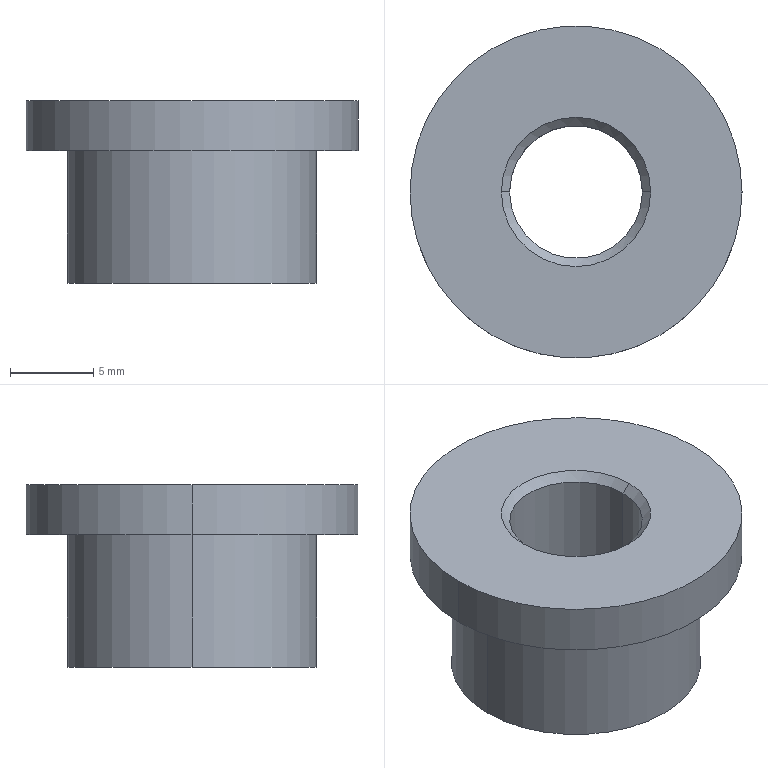Part | SolidWorks | features Chamfer 1, Extrusion 1, ICE 1 | 1 solid | 13 faces | box 20 x 20 x 11 mm | volume 1797 mm3 | cylinder 6 | cone 4 | plane 3 | commonest cylinder face diameters 8 x2 15 x2 20 x2
STEP:
#1=CARTESIAN_POINT('',(141.505,180.569,2.5));
#2=VERTEX_POINT('',#1);
#3=CARTESIAN_POINT('',(149.505,180.569,2.5));
#4=VERTEX_POINT('',#3);
#5=CARTESIAN_POINT('',(145.505,180.569,2.5));
#6=DIRECTION('',(0.,0.,1.));
#7=DIRECTION('',(1.,0.,0.));
#8=AXIS2_PLACEMENT_3D('',#5,#6,#7);
#9=CIRCLE('',#8,4.);
#10=EDGE_CURVE('',#2,#4,#9,.T.);
#11=ORIENTED_EDGE('',*,*,#10,.F.);
#12=CARTESIAN_POINT('',(141.005,180.569,3.));
#13=VERTEX_POINT('',#12);
#14=CARTESIAN_POINT('',(141.505,180.569,2.5));
#15=DIRECTION('',(-0.7071,0.,0.7071));
#16=VECTOR('',#15,1000.);
#17=LINE('',#14,#16);
#18=EDGE_CURVE('',#2,#13,#17,.T.);
#19=ORIENTED_EDGE('',*,*,#18,.T.);
#20=CARTESIAN_POINT('',(150.005,180.569,3.));
#21=VERTEX_POINT('',#20);
#22=CARTESIAN_POINT('',(145.505,180.569,3.));
#23=DIRECTION('',(0.,0.,-1.));
#24=DIRECTION('',(1.,0.,0.));
#25=AXIS2_PLACEMENT_3D('',#22,#23,#24);
#26=CIRCLE('',#25,4.5);
#27=EDGE_CURVE('',#21,#13,#26,.T.);
#28=ORIENTED_EDGE('',*,*,#27,.F.);
#29=CARTESIAN_POINT('',(149.505,180.569,2.5));
#30=DIRECTION('',(0.7071,0.,0.7071));
#31=VECTOR('',#30,1000.);
#32=LINE('',#29,#31);
#33=EDGE_CURVE('',#4,#21,#32,.T.);
#34=ORIENTED_EDGE('',*,*,#33,.F.);
#35=EDGE_LOOP('',(#11,#19,#28,#34));
#36=FACE_OUTER_BOUND('',#35,.T.);
#37=CARTESIAN_POINT('',(145.505,180.569,2.5));
#38=DIRECTION('',(0.,0.,1.));
#39=DIRECTION('',(1.,0.,0.));
#40=AXIS2_PLACEMENT_3D('',#37,#38,#39);
#41=CONICAL_SURFACE('',#40,4.,0.7854);
#42=ADVANCED_FACE('',(#36),#41,.F.);
#43=CARTESIAN_POINT('',(149.505,180.569,-7.5));
#44=VERTEX_POINT('',#43);
#45=CARTESIAN_POINT('',(141.505,180.569,-7.5));
#46=VERTEX_POINT('',#45);
#47=CARTESIAN_POINT('',(145.505,180.569,-7.5));
#48=DIRECTION('',(0.,0.,-1.));
#49=DIRECTION('',(1.,0.,0.));
#50=AXIS2_PLACEMENT_3D('',#47,#48,#49);
#51=CIRCLE('',#50,4.);
#52=EDGE_CURVE('',#44,#46,#51,.T.);
#53=ORIENTED_EDGE('',*,*,#52,.F.);
#54=CARTESIAN_POINT('',(150.005,180.569,-8.));
#55=VERTEX_POINT('',#54);
#56=CARTESIAN_POINT('',(149.505,180.569,-7.5));
#57=DIRECTION('',(0.7071,0.,-0.7071));
#58=VECTOR('',#57,1000.);
#59=LINE('',#56,#58);
#60=EDGE_CURVE('',#44,#55,#59,.T.);
#61=ORIENTED_EDGE('',*,*,#60,.T.);
#62=CARTESIAN_POINT('',(141.005,180.569,-8.));
#63=VERTEX_POINT('',#62);
#64=CARTESIAN_POINT('',(145.505,180.569,-8.));
#65=DIRECTION('',(0.,0.,1.));
#66=DIRECTION('',(1.,0.,0.));
#67=AXIS2_PLACEMENT_3D('',#64,#65,#66);
#68=CIRCLE('',#67,4.5);
#69=EDGE_CURVE('',#63,#55,#68,.T.);
#70=ORIENTED_EDGE('',*,*,#69,.F.);
#71=CARTESIAN_POINT('',(141.505,180.569,-7.5));
#72=DIRECTION('',(-0.7071,0.,-0.7071));
#73=VECTOR('',#72,1000.);
#74=LINE('',#71,#73);
#75=EDGE_CURVE('',#46,#63,#74,.T.);
#76=ORIENTED_EDGE('',*,*,#75,.F.);
#77=EDGE_LOOP('',(#53,#61,#70,#76));
#78=FACE_OUTER_BOUND('',#77,.T.);
#79=CARTESIAN_POINT('',(145.505,180.569,-7.5));
#80=DIRECTION('',(0.,0.,-1.));
#81=DIRECTION('',(-1.,0.,0.));
#82=AXIS2_PLACEMENT_3D('',#79,#80,#81);
#83=CONICAL_SURFACE('',#82,4.,0.7854);
#84=ADVANCED_FACE('',(#78),#83,.F.);
#85=CARTESIAN_POINT('',(155.505,180.569,3.));
#86=VERTEX_POINT('',#85);
#87=CARTESIAN_POINT('',(135.505,180.569,3.));
#88=VERTEX_POINT('',#87);
#89=CARTESIAN_POINT('',(145.505,180.569,3.));
#90=DIRECTION('',(0.,0.,1.));
#91=DIRECTION('',(1.,0.,0.));
#92=AXIS2_PLACEMENT_3D('',#89,#90,#91);
#93=CIRCLE('',#92,10.);
#94=EDGE_CURVE('',#86,#88,#93,.T.);
#95=ORIENTED_EDGE('',*,*,#94,.F.);
#96=CARTESIAN_POINT('',(155.505,180.569,0.));
#97=VERTEX_POINT('',#96);
#98=CARTESIAN_POINT('',(155.505,180.569,3.));
#99=DIRECTION('',(0.,0.,-1.));
#100=VECTOR('',#99,1000.);
#101=LINE('',#98,#100);
#102=EDGE_CURVE('',#86,#97,#101,.T.);
#103=ORIENTED_EDGE('',*,*,#102,.T.);
#104=CARTESIAN_POINT('',(135.505,180.569,0.));
#105=VERTEX_POINT('',#104);
#106=CARTESIAN_POINT('',(145.505,180.569,0.));
#107=DIRECTION('',(0.,0.,1.));
#108=DIRECTION('',(1.,0.,0.));
#109=AXIS2_PLACEMENT_3D('',#106,#107,#108);
#110=CIRCLE('',#109,10.);
#111=EDGE_CURVE('',#97,#105,#110,.T.);
#112=ORIENTED_EDGE('',*,*,#111,.T.);
#113=CARTESIAN_POINT('',(135.505,180.569,3.));
#114=DIRECTION('',(0.,0.,-1.));
#115=VECTOR('',#114,1000.);
#116=LINE('',#113,#115);
#117=EDGE_CURVE('',#88,#105,#116,.T.);
#118=ORIENTED_EDGE('',*,*,#117,.F.);
#119=EDGE_LOOP('',(#95,#103,#112,#118));
#120=FACE_OUTER_BOUND('',#119,.T.);
#121=CARTESIAN_POINT('',(145.505,180.569,3.));
#122=DIRECTION('',(0.,0.,-1.));
#123=DIRECTION('',(-1.,0.,0.));
#124=AXIS2_PLACEMENT_3D('',#121,#122,#123);
#125=CYLINDRICAL_SURFACE('',#124,10.);
#126=ADVANCED_FACE('',(#120),#125,.T.);
#127=ORIENTED_EDGE('',*,*,#52,.T.);
#128=CARTESIAN_POINT('',(141.505,180.569,-29.213));
#129=DIRECTION('',(0.,0.,1.));
#130=VECTOR('',#129,1000.);
#131=LINE('',#128,#130);
#132=EDGE_CURVE('',#46,#2,#131,.T.);
#133=ORIENTED_EDGE('',*,*,#132,.T.);
#134=ORIENTED_EDGE('',*,*,#10,.T.);
#135=CARTESIAN_POINT('',(149.505,180.569,-29.213));
#136=DIRECTION('',(0.,0.,1.));
#137=VECTOR('',#136,1000.);
#138=LINE('',#135,#137);
#139=EDGE_CURVE('',#44,#4,#138,.T.);
#140=ORIENTED_EDGE('',*,*,#139,.F.);
#141=EDGE_LOOP('',(#127,#133,#134,#140));
#142=FACE_OUTER_BOUND('',#141,.T.);
#143=CARTESIAN_POINT('',(145.505,180.569,-29.213));
#144=DIRECTION('',(0.,0.,1.));
#145=DIRECTION('',(1.,0.,0.));
#146=AXIS2_PLACEMENT_3D('',#143,#144,#145);
#147=CYLINDRICAL_SURFACE('',#146,4.);
#148=ADVANCED_FACE('',(#142),#147,.F.);
#149=CARTESIAN_POINT('',(138.005,180.569,-8.));
#150=VERTEX_POINT('',#149);
#151=CARTESIAN_POINT('',(153.005,180.569,-8.));
#152=VERTEX_POINT('',#151);
#153=CARTESIAN_POINT('',(145.505,180.569,-8.));
#154=DIRECTION('',(0.,0.,-1.));
#155=DIRECTION('',(1.,0.,0.));
#156=AXIS2_PLACEMENT_3D('',#153,#154,#155);
#157=CIRCLE('',#156,7.5);
#158=EDGE_CURVE('',#150,#152,#157,.T.);
#159=ORIENTED_EDGE('',*,*,#158,.F.);
#160=CARTESIAN_POINT('',(138.005,180.569,0.));
#161=VERTEX_POINT('',#160);
#162=CARTESIAN_POINT('',(138.005,180.569,-29.213));
#163=DIRECTION('',(0.,0.,1.));
#164=VECTOR('',#163,1000.);
#165=LINE('',#162,#164);
#166=EDGE_CURVE('',#150,#161,#165,.T.);
#167=ORIENTED_EDGE('',*,*,#166,.T.);
#168=CARTESIAN_POINT('',(153.005,180.569,0.));
#169=VERTEX_POINT('',#168);
#170=CARTESIAN_POINT('',(145.505,180.569,0.));
#171=DIRECTION('',(0.,0.,1.));
#172=DIRECTION('',(1.,0.,0.));
#173=AXIS2_PLACEMENT_3D('',#170,#171,#172);
#174=CIRCLE('',#173,7.5);
#175=EDGE_CURVE('',#169,#161,#174,.T.);
#176=ORIENTED_EDGE('',*,*,#175,.F.);
#177=CARTESIAN_POINT('',(153.005,180.569,-29.213));
#178=DIRECTION('',(0.,0.,1.));
#179=VECTOR('',#178,1000.);
#180=LINE('',#177,#179);
#181=EDGE_CURVE('',#152,#169,#180,.T.);
#182=ORIENTED_EDGE('',*,*,#181,.F.);
#183=EDGE_LOOP('',(#159,#167,#176,#182));
#184=FACE_OUTER_BOUND('',#183,.T.);
#185=CARTESIAN_POINT('',(145.505,180.569,-29.213));
#186=DIRECTION('',(0.,0.,1.));
#187=DIRECTION('',(1.,0.,0.));
#188=AXIS2_PLACEMENT_3D('',#185,#186,#187);
#189=CYLINDRICAL_SURFACE('',#188,7.5);
#190=ADVANCED_FACE('',(#184),#189,.T.);
#191=ORIENTED_EDGE('',*,*,#166,.F.);
#192=CARTESIAN_POINT('',(145.505,180.569,-8.));
#193=DIRECTION('',(0.,0.,-1.));
#194=DIRECTION('',(1.,0.,0.));
#195=AXIS2_PLACEMENT_3D('',#192,#193,#194);
#196=CIRCLE('',#195,7.5);
#197=EDGE_CURVE('',#152,#150,#196,.T.);
#198=ORIENTED_EDGE('',*,*,#197,.F.);
#199=ORIENTED_EDGE('',*,*,#181,.T.);
#200=CARTESIAN_POINT('',(145.505,180.569,0.));
#201=DIRECTION('',(0.,0.,1.));
#202=DIRECTION('',(1.,0.,0.));
#203=AXIS2_PLACEMENT_3D('',#200,#201,#202);
#204=CIRCLE('',#203,7.5);
#205=EDGE_CURVE('',#161,#169,#204,.T.);
#206=ORIENTED_EDGE('',*,*,#205,.F.);
#207=EDGE_LOOP('',(#191,#198,#199,#206));
#208=FACE_OUTER_BOUND('',#207,.T.);
#209=CARTESIAN_POINT('',(145.505,180.569,-29.213));
#210=DIRECTION('',(0.,0.,1.));
#211=DIRECTION('',(1.,0.,0.));
#212=AXIS2_PLACEMENT_3D('',#209,#210,#211);
#213=CYLINDRICAL_SURFACE('',#212,7.5);
#214=ADVANCED_FACE('',(#208),#213,.T.);
#215=ORIENTED_EDGE('',*,*,#132,.F.);
#216=CARTESIAN_POINT('',(145.505,180.569,-7.5));
#217=DIRECTION('',(0.,0.,-1.));
#218=DIRECTION('',(1.,0.,0.));
#219=AXIS2_PLACEMENT_3D('',#216,#217,#218);
#220=CIRCLE('',#219,4.);
#221=EDGE_CURVE('',#46,#44,#220,.T.);
#222=ORIENTED_EDGE('',*,*,#221,.T.);
#223=ORIENTED_EDGE('',*,*,#139,.T.);
#224=CARTESIAN_POINT('',(145.505,180.569,2.5));
#225=DIRECTION('',(0.,0.,1.));
#226=DIRECTION('',(1.,0.,0.));
#227=AXIS2_PLACEMENT_3D('',#224,#225,#226);
#228=CIRCLE('',#227,4.);
#229=EDGE_CURVE('',#4,#2,#228,.T.);
#230=ORIENTED_EDGE('',*,*,#229,.T.);
#231=EDGE_LOOP('',(#215,#222,#223,#230));
#232=FACE_OUTER_BOUND('',#231,.T.);
#233=CARTESIAN_POINT('',(145.505,180.569,-29.213));
#234=DIRECTION('',(0.,0.,1.));
#235=DIRECTION('',(1.,0.,0.));
#236=AXIS2_PLACEMENT_3D('',#233,#234,#235);
#237=CYLINDRICAL_SURFACE('',#236,4.);
#238=ADVANCED_FACE('',(#232),#237,.F.);
#239=ORIENTED_EDGE('',*,*,#69,.T.);
#240=CARTESIAN_POINT('',(145.505,180.569,-8.));
#241=DIRECTION('',(0.,0.,1.));
#242=DIRECTION('',(1.,0.,0.));
#243=AXIS2_PLACEMENT_3D('',#240,#241,#242);
#244=CIRCLE('',#243,4.5);
#245=EDGE_CURVE('',#55,#63,#244,.T.);
#246=ORIENTED_EDGE('',*,*,#245,.T.);
#247=EDGE_LOOP('',(#239,#246));
#248=FACE_BOUND('',#247,.T.);
#249=ORIENTED_EDGE('',*,*,#197,.T.);
#250=ORIENTED_EDGE('',*,*,#158,.T.);
#251=EDGE_LOOP('',(#249,#250));
#252=FACE_OUTER_BOUND('',#251,.T.);
#253=CARTESIAN_POINT('',(0.,0.,-8.));
#254=DIRECTION('',(0.,0.,1.));
#255=DIRECTION('',(1.,0.,0.));
#256=AXIS2_PLACEMENT_3D('',#253,#254,#255);
#257=PLANE('',#256);
#258=ADVANCED_FACE('',(#248,#252),#257,.F.);
#259=ORIENTED_EDGE('',*,*,#27,.T.);
#260=CARTESIAN_POINT('',(145.505,180.569,3.));
#261=DIRECTION('',(0.,0.,-1.));
#262=DIRECTION('',(1.,0.,0.));
#263=AXIS2_PLACEMENT_3D('',#260,#261,#262);
#264=CIRCLE('',#263,4.5);
#265=EDGE_CURVE('',#13,#21,#264,.T.);
#266=ORIENTED_EDGE('',*,*,#265,.T.);
#267=EDGE_LOOP('',(#259,#266));
#268=FACE_BOUND('',#267,.T.);
#269=CARTESIAN_POINT('',(145.505,180.569,3.));
#270=DIRECTION('',(0.,0.,1.));
#271=DIRECTION('',(1.,0.,0.));
#272=AXIS2_PLACEMENT_3D('',#269,#270,#271);
#273=CIRCLE('',#272,10.);
#274=EDGE_CURVE('',#88,#86,#273,.T.);
#275=ORIENTED_EDGE('',*,*,#274,.T.);
#276=ORIENTED_EDGE('',*,*,#94,.T.);
#277=EDGE_LOOP('',(#275,#276));
#278=FACE_OUTER_BOUND('',#277,.T.);
#279=CARTESIAN_POINT('',(145.505,180.569,3.));
#280=DIRECTION('',(0.,0.,1.));
#281=DIRECTION('',(1.,0.,0.));
#282=AXIS2_PLACEMENT_3D('',#279,#280,#281);
#283=PLANE('',#282);
#284=ADVANCED_FACE('',(#268,#278),#283,.T.);
#285=ORIENTED_EDGE('',*,*,#175,.T.);
#286=ORIENTED_EDGE('',*,*,#205,.T.);
#287=EDGE_LOOP('',(#285,#286));
#288=FACE_BOUND('',#287,.T.);
#289=CARTESIAN_POINT('',(145.505,180.569,0.));
#290=DIRECTION('',(0.,0.,1.));
#291=DIRECTION('',(1.,0.,0.));
#292=AXIS2_PLACEMENT_3D('',#289,#290,#291);
#293=CIRCLE('',#292,10.);
#294=EDGE_CURVE('',#105,#97,#293,.T.);
#295=ORIENTED_EDGE('',*,*,#294,.F.);
#296=ORIENTED_EDGE('',*,*,#111,.F.);
#297=EDGE_LOOP('',(#295,#296));
#298=FACE_OUTER_BOUND('',#297,.T.);
#299=CARTESIAN_POINT('',(145.505,180.569,0.));
#300=DIRECTION('',(0.,0.,1.));
#301=DIRECTION('',(1.,0.,0.));
#302=AXIS2_PLACEMENT_3D('',#299,#300,#301);
#303=PLANE('',#302);
#304=ADVANCED_FACE('',(#288,#298),#303,.F.);
#305=ORIENTED_EDGE('',*,*,#102,.F.);
#306=ORIENTED_EDGE('',*,*,#274,.F.);
#307=ORIENTED_EDGE('',*,*,#117,.T.);
#308=ORIENTED_EDGE('',*,*,#294,.T.);
#309=EDGE_LOOP('',(#305,#306,#307,#308));
#310=FACE_OUTER_BOUND('',#309,.T.);
#311=CARTESIAN_POINT('',(145.505,180.569,3.));
#312=DIRECTION('',(0.,0.,-1.));
#313=DIRECTION('',(-1.,0.,0.));
#314=AXIS2_PLACEMENT_3D('',#311,#312,#313);
#315=CYLINDRICAL_SURFACE('',#314,10.);
#316=ADVANCED_FACE('',(#310),#315,.T.);
#317=ORIENTED_EDGE('',*,*,#60,.F.);
#318=ORIENTED_EDGE('',*,*,#221,.F.);
#319=ORIENTED_EDGE('',*,*,#75,.T.);
#320=ORIENTED_EDGE('',*,*,#245,.F.);
#321=EDGE_LOOP('',(#317,#318,#319,#320));
#322=FACE_OUTER_BOUND('',#321,.T.);
#323=CARTESIAN_POINT('',(145.505,180.569,-7.5));
#324=DIRECTION('',(0.,0.,-1.));
#325=DIRECTION('',(-1.,0.,0.));
#326=AXIS2_PLACEMENT_3D('',#323,#324,#325);
#327=CONICAL_SURFACE('',#326,4.,0.7854);
#328=ADVANCED_FACE('',(#322),#327,.F.);
#329=ORIENTED_EDGE('',*,*,#18,.F.);
#330=ORIENTED_EDGE('',*,*,#229,.F.);
#331=ORIENTED_EDGE('',*,*,#33,.T.);
#332=ORIENTED_EDGE('',*,*,#265,.F.);
#333=EDGE_LOOP('',(#329,#330,#331,#332));
#334=FACE_OUTER_BOUND('',#333,.T.);
#335=CARTESIAN_POINT('',(145.505,180.569,2.5));
#336=DIRECTION('',(0.,0.,1.));
#337=DIRECTION('',(1.,0.,0.));
#338=AXIS2_PLACEMENT_3D('',#335,#336,#337);
#339=CONICAL_SURFACE('',#338,4.,0.7854);
#340=ADVANCED_FACE('',(#334),#339,.F.);
#341=CLOSED_SHELL('',(#42,#84,#126,#148,#190,#214,#238,#258,#284,#304,#316,#328,#340));
#342=MANIFOLD_SOLID_BREP('',#341);
#343=CARTESIAN_POINT('',(0.,0.,0.));
#344=DIRECTION('',(0.,0.,1.));
#345=DIRECTION('',(1.,0.,0.));
#346=AXIS2_PLACEMENT_3D('',#343,#344,#345);
#347=(LENGTH_UNIT()NAMED_UNIT(*)SI_UNIT(.MILLI.,.METRE.));
#348=UNCERTAINTY_MEASURE_WITH_UNIT(LENGTH_MEASURE(0.00001),#347,'','');
#349=(NAMED_UNIT(*)PLANE_ANGLE_UNIT()SI_UNIT($,.RADIAN.));
#350=(NAMED_UNIT(*)SI_UNIT($,.STERADIAN.)SOLID_ANGLE_UNIT());
#351=(GEOMETRIC_REPRESENTATION_CONTEXT(3)GLOBAL_UNCERTAINTY_ASSIGNED_CONTEXT((#348))GLOBAL_UNIT_ASSIGNED_CONTEXT((#347,#349,#350))REPRESENTATION_CONTEXT('',''));
#352=ADVANCED_BREP_SHAPE_REPRESENTATION('',(#342,#346),#351);